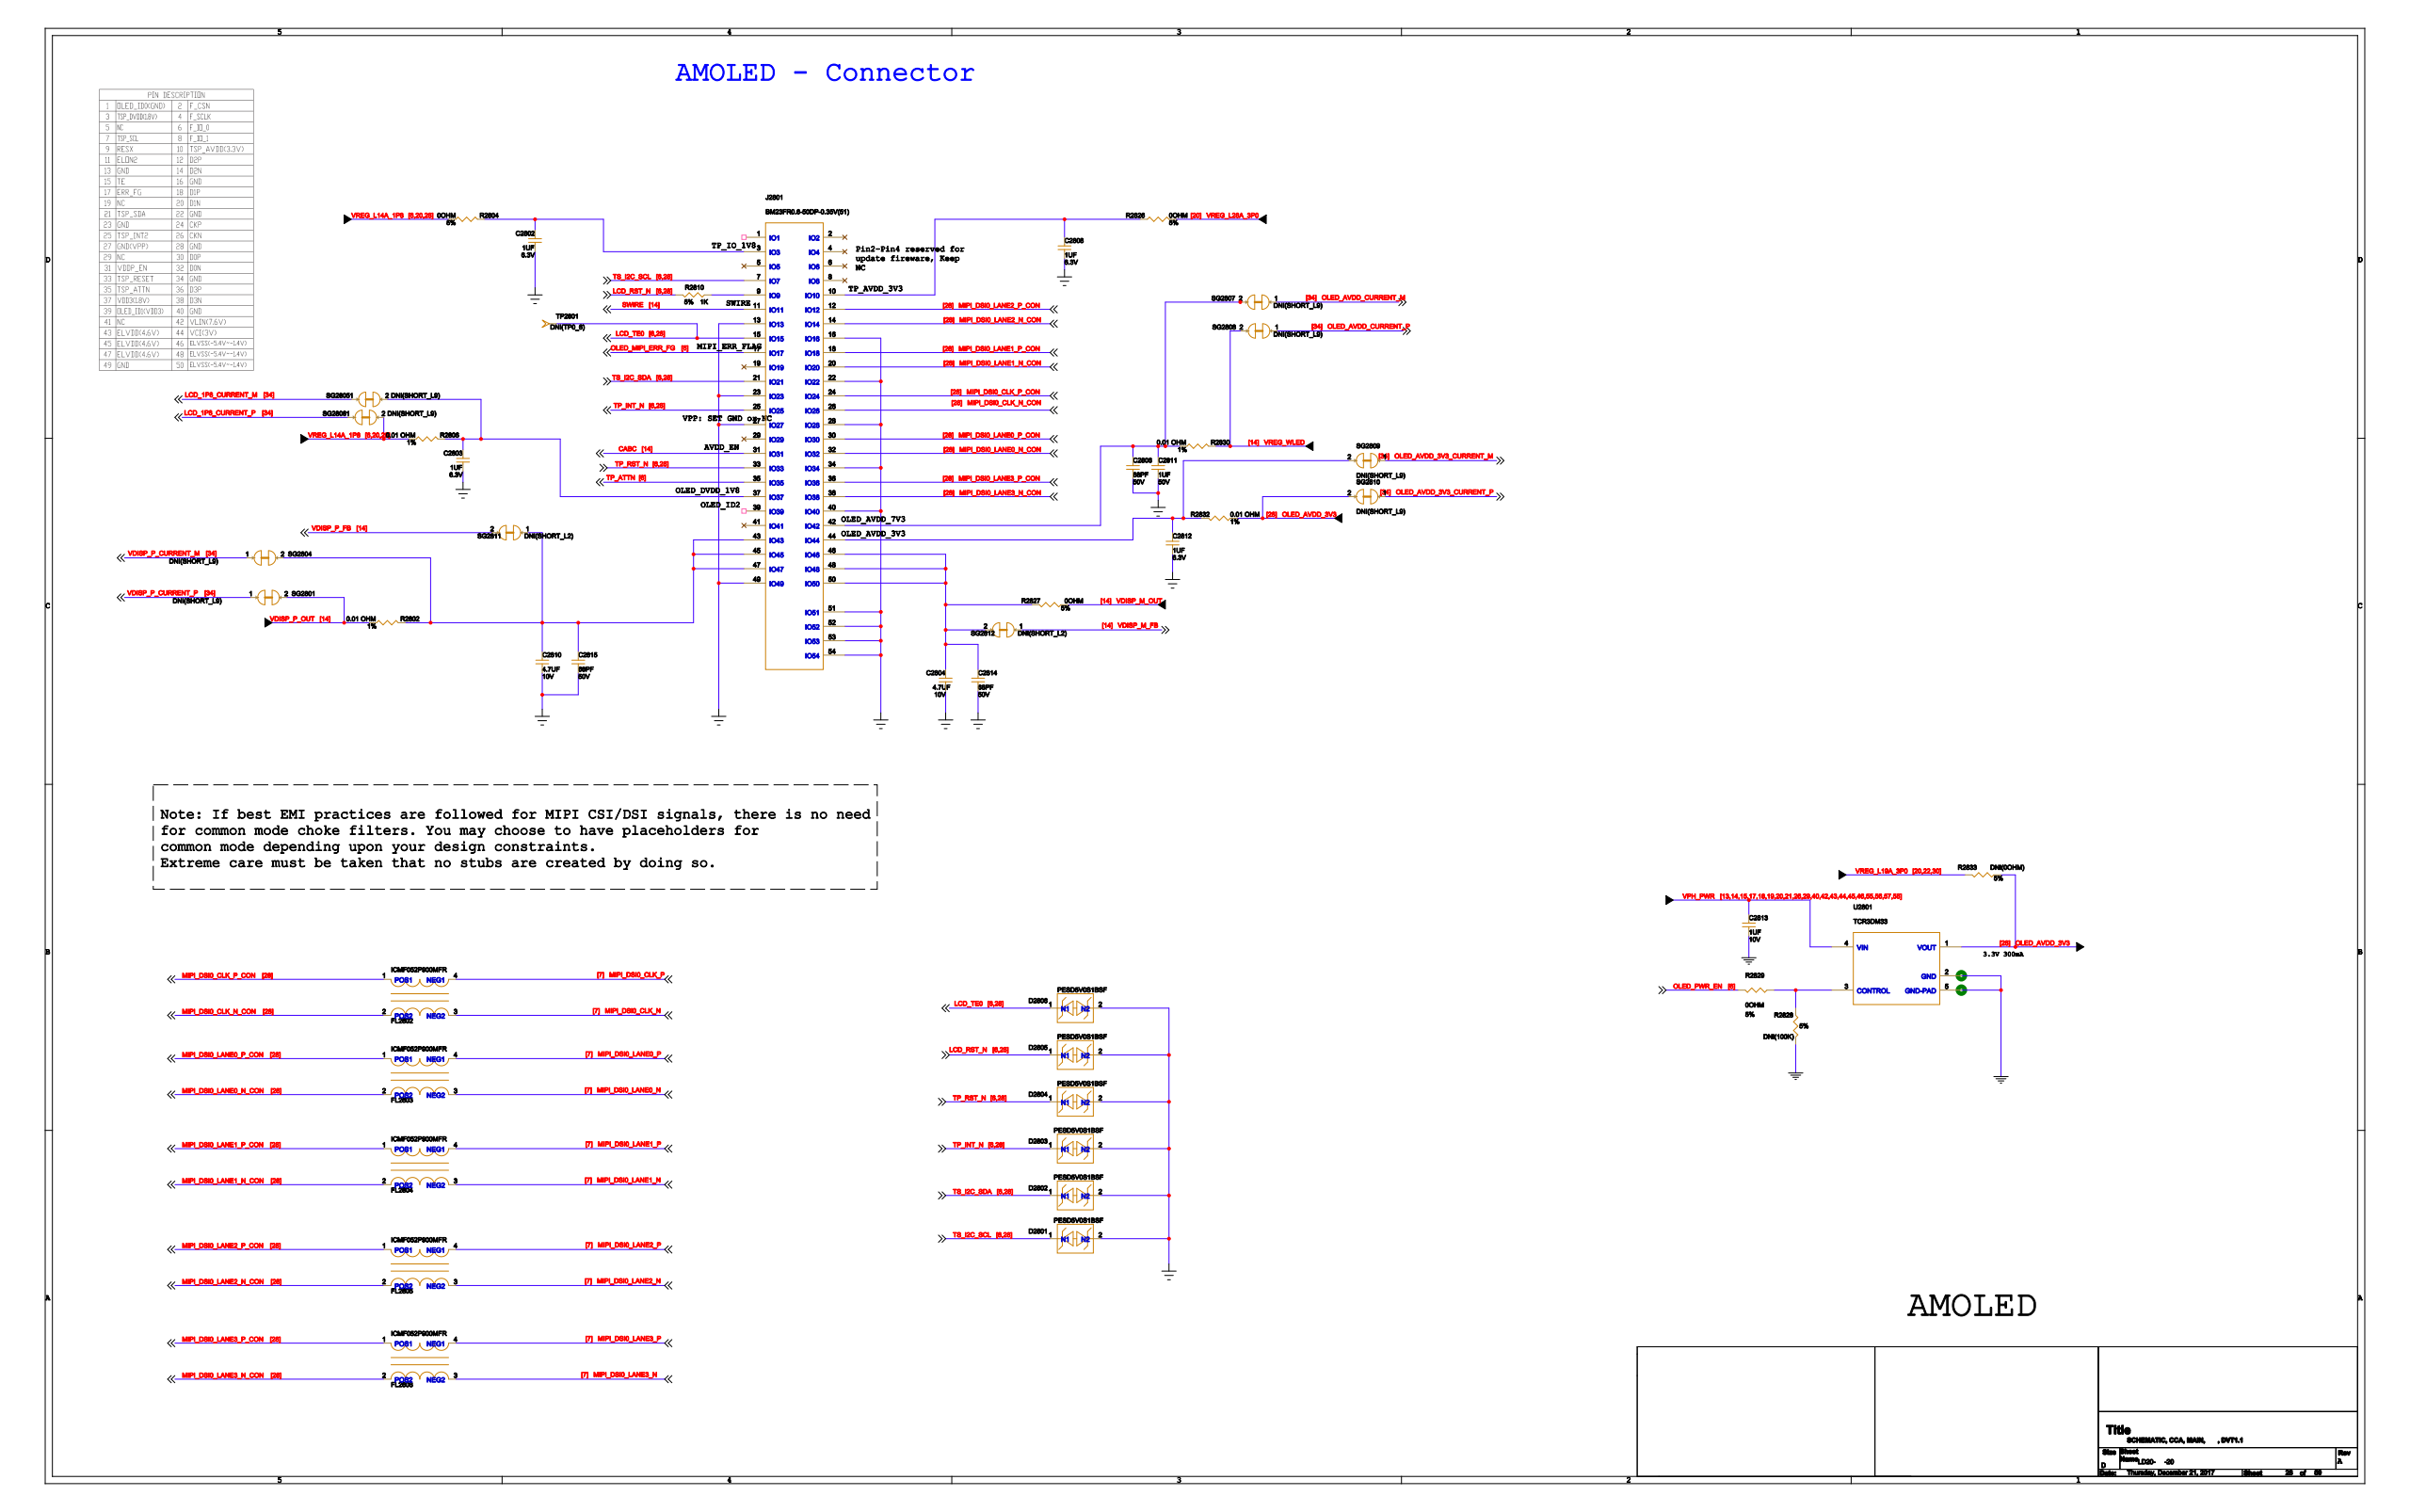Circuit board | Cadence Allegro | 1520 parts | 1149 nets | one sheet of the schematic
Parts on this sheet (reference | value | footprint):
C2802 | 1UF | 2P0201R
C2803 | 1UF | 2P0201R
C2804 | 4.7UF | 2P0402R
C2806 | 68PF | 2P0201R
C2808 | 1UF | 2P0201R
C2810 | 4.7UF | 2P0402R
C2811 | 1UF | 2P0603R
C2812 | 1UF | 2P0201R
C2813 | 1UF | 2P0402R
C2814 | 68PF | 2P0201R
C2815 | 68PF | 2P0201R
D2801 | PESD5V0S1BSF | 2PSM25X13N
D2802 | PESD5V0S1BSF | 2PSM25X13N
D2803 | PESD5V0S1BSF | 2PSM25X13N
D2804 | PESD5V0S1BSF | 2PSM25X13N
D2805 | PESD5V0S1BSF | 2PSM25X13N
D2806 | PESD5V0S1BSF | 2PSM25X13N
FL2802 | ICMF052P900MFR | ICMF052P900MFR
FL2803 | ICMF052P900MFR | ICMF052P900MFR
FL2804 | ICMF052P900MFR | ICMF052P900MFR
FL2805 | ICMF052P900MFR | ICMF052P900MFR
FL2808 | ICMF052P900MFR | ICMF052P900MFR
J2801 | BM23FR0.6-50DP-0.35V(51) | 54PCONS138
R2802 | 0.01 OHM | 2P0603R
R2804 | 0OHM | 2P0201R
R2806 | 0.01 OHM | 2P0603R
R2810 | 1K | 2P0201R
R2826 | 0OHM | 2P0201R
R2827 | 0OHM | 2P0201R
R2828 | DNI(100K) | 2P0201R_DNI
R2829 | 0OHM | 2P0201R
R2830 | 0.01 OHM | 2P0603R
R2832 | 0.01 OHM | 2P0603R
R2833 | DNI(0OHM) | 2P0201R_DNI
SG2801 | DNI(SHORT_L9) | SHORT_L9_2REC08X12
SG2804 | DNI(SHORT_L9) | SHORT_L9_2REC08X12
SG2807 | DNI(SHORT_L9) | SHORT_L9_2REC08X12
SG2808 | DNI(SHORT_L9) | SHORT_L9_2REC08X12
SG2809 | DNI(SHORT_L9) | SHORT_L9_2REC08X12
SG2810 | DNI(SHORT_L9) | SHORT_L9_2REC08X12
SG2811 | DNI(SHORT_L2) | SHORT_L2_2REC08X12
SG2812 | DNI(SHORT_L2) | SHORT_L2_2REC08X12
TP2801 | DNI(TP0_6) | TP-0_6
U2801 | TCR3DM33 | 5PSM41X41NV1
Nets of these parts (net: part-pin ...):
GND: C2802-2 C2803-2 C2804-2 C2806-2 C2808-2 C2810-2 C2811-2 C2812-2 C2813-2 C2814-2 C2815-2 D2801-2 D2802-2 D2803-2 D2804-2 D2805-2 D2806-2 R2828-1 U2801-2 U2801-5 J2801-13 J2801-16 J2801-22 J2801-23 J2801-27 J2801-28 J2801-34 J2801-40 J2801-49 J2801-51 J2801-52 J2801-53 J2801-54
VREG_L19A_3P0: R2833-1
VPH_PWR: C2813-1 U2801-4
N49237624: C2810-1 C2815-1 R2802-2 SG2804-2 SG2811-1 J2801-43 J2801-45 J2801-47
VDISP_P_FB: SG2811-2
VDISP_M_FB: SG2812-1
N49239771: C2804-1 C2814-1 R2827-1 SG2812-2 J2801-46 J2801-48 J2801-50
VDISP_P_CURRENT_P: SG2801-1
VDISP_P_OUT: R2802-1 SG2801-2
VDISP_P_CURRENT_M: SG2804-1
N49238155: C2803-1 R2806-2 J2801-37
VREG_L14A_1P8: R2804-1 R2806-1
OLED_AVDD_CURRENT_M: SG2807-1
N49239755: C2806-1 C2811-1 R2830-1 SG2807-2 J2801-42
OLED_AVDD_CURRENT_P: SG2808-1
VREG_WLED: R2830-2 SG2808-2
OLED_AVDD_3V3_CURRENT_M: SG2809-1
N49239742: C2812-1 R2832-1 SG2809-2 J2801-44
OLED_AVDD_3V3_CURRENT_P: SG2810-1
OLED_AVDD_3V3: R2832-2 R2833-2 SG2810-2 U2801-1
N49239973: C2808-1 R2826-2 J2801-10
SWIRE: J2801-11
MIPI_DSI0_LANE2_P_CON: FL2805-1 J2801-12
MIPI_DSI0_LANE2_N_CON: FL2805-2 J2801-14
LCD_TE0: D2806-1 TP2801-1 J2801-15
OLED_MIPI_ERR_FG: J2801-17
MIPI_DSI0_LANE1_P_CON: FL2804-1 J2801-18
MIPI_DSI0_LANE1_N_CON: FL2804-2 J2801-20
TS_I2C_SDA: D2802-1 J2801-21
MIPI_DSI0_CLK_P_CON: FL2802-1 J2801-24
TP_INT_N: D2803-1 J2801-25
MIPI_DSI0_CLK_N_CON: FL2802-2 J2801-26
N49236512: C2802-1 R2804-2 J2801-3
MIPI_DSI0_LANE0_P_CON: FL2803-1 J2801-30
CABC: J2801-31
MIPI_DSI0_LANE0_N_CON: FL2803-2 J2801-32
TP_RST_N: D2804-1 J2801-33
TP_ATTN: J2801-35
MIPI_DSI0_LANE3_P_CON: FL2808-1 J2801-36
MIPI_DSI0_LANE3_N_CON: FL2808-2 J2801-38
TS_I2C_SCL: D2801-1 J2801-7
N49236802: R2810-1 J2801-9
LCD_RST_N: D2805-1 R2810-2
VREG_L28A_3P0: R2826-1
VDISP_M_OUT: R2827-2
OLED_PWR_EN: R2829-1
N49632201: R2828-2 R2829-2 U2801-3
MIPI_DSI0_CLK_P: FL2802-4
MIPI_DSI0_CLK_N: FL2802-3
MIPI_DSI0_LANE0_P: FL2803-4
MIPI_DSI0_LANE0_N: FL2803-3
MIPI_DSI0_LANE1_P: FL2804-4
MIPI_DSI0_LANE1_N: FL2804-3
MIPI_DSI0_LANE2_P: FL2805-4
MIPI_DSI0_LANE2_N: FL2805-3
MIPI_DSI0_LANE3_P: FL2808-4
MIPI_DSI0_LANE3_N: FL2808-3